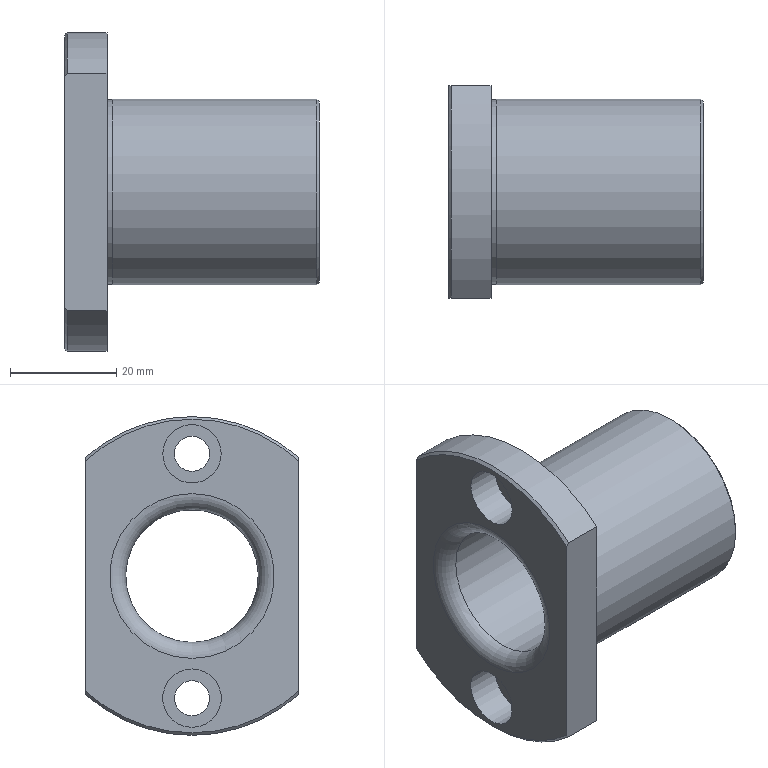Part | NX | features bushing 2 | 1 solid | 21 faces | box 48 x 40 x 60 mm | volume 31044 mm3 | cylinder 9 | plane 8 | cone 3 | torus 1 | commonest cylinder face diameters 6.6 x2 11 x2 60 x2 25 x1 34.65 x1 35 x1
STEP:
#1=CARTESIAN_POINT('',(-1.5,0.,-28.5));
#2=VERTEX_POINT('',#1);
#3=CARTESIAN_POINT('',(-1.5,0.,-23.));
#4=DIRECTION('',(1.,0.,0.));
#5=DIRECTION('',(0.,0.,-1.));
#6=AXIS2_PLACEMENT_3D('',#3,#4,#5);
#7=CIRCLE('',#6,5.5);
#8=EDGE_CURVE('',#2,#2,#7,.F.);
#9=ORIENTED_EDGE('',*,*,#8,.F.);
#10=EDGE_LOOP('',(#9));
#11=FACE_BOUND('',#10,.T.);
#12=CARTESIAN_POINT('',(-8.,0.,-28.5));
#13=VERTEX_POINT('',#12);
#14=CARTESIAN_POINT('',(-8.,0.,-23.));
#15=DIRECTION('',(1.,0.,0.));
#16=DIRECTION('',(0.,0.,-1.));
#17=AXIS2_PLACEMENT_3D('',#14,#15,#16);
#18=CIRCLE('',#17,5.5);
#19=EDGE_CURVE('',#13,#13,#18,.T.);
#20=ORIENTED_EDGE('',*,*,#19,.F.);
#21=EDGE_LOOP('',(#20));
#22=FACE_BOUND('',#21,.T.);
#23=CARTESIAN_POINT('',(-8.,0.,-23.));
#24=DIRECTION('',(1.,0.,0.));
#25=DIRECTION('',(0.,0.,-1.));
#26=AXIS2_PLACEMENT_3D('',#23,#24,#25);
#27=CYLINDRICAL_SURFACE('',#26,5.5);
#28=ADVANCED_FACE('',(#11,#22),#27,.F.);
#29=CARTESIAN_POINT('',(-1.5,5.5,23.));
#30=VERTEX_POINT('',#29);
#31=CARTESIAN_POINT('',(-1.5,0.,23.));
#32=DIRECTION('',(1.,0.,0.));
#33=DIRECTION('',(0.,1.,0.));
#34=AXIS2_PLACEMENT_3D('',#31,#32,#33);
#35=CIRCLE('',#34,5.5);
#36=EDGE_CURVE('',#30,#30,#35,.F.);
#37=ORIENTED_EDGE('',*,*,#36,.F.);
#38=EDGE_LOOP('',(#37));
#39=FACE_BOUND('',#38,.T.);
#40=CARTESIAN_POINT('',(-8.,5.5,23.));
#41=VERTEX_POINT('',#40);
#42=CARTESIAN_POINT('',(-8.,0.,23.));
#43=DIRECTION('',(1.,0.,0.));
#44=DIRECTION('',(0.,1.,0.));
#45=AXIS2_PLACEMENT_3D('',#42,#43,#44);
#46=CIRCLE('',#45,5.5);
#47=EDGE_CURVE('',#41,#41,#46,.T.);
#48=ORIENTED_EDGE('',*,*,#47,.F.);
#49=EDGE_LOOP('',(#48));
#50=FACE_BOUND('',#49,.T.);
#51=CARTESIAN_POINT('',(-8.,0.,23.));
#52=DIRECTION('',(1.,0.,0.));
#53=DIRECTION('',(0.,1.,0.));
#54=AXIS2_PLACEMENT_3D('',#51,#52,#53);
#55=CYLINDRICAL_SURFACE('',#54,5.5);
#56=ADVANCED_FACE('',(#39,#50),#55,.F.);
#57=CARTESIAN_POINT('',(-8.,-20.,21.685));
#58=VERTEX_POINT('',#57);
#59=CARTESIAN_POINT('',(-8.,20.,21.685));
#60=VERTEX_POINT('',#59);
#61=CARTESIAN_POINT('',(-8.,0.,0.));
#62=DIRECTION('',(-1.,0.,0.));
#63=DIRECTION('',(0.,0.,1.));
#64=AXIS2_PLACEMENT_3D('',#61,#62,#63);
#65=CIRCLE('',#64,29.5);
#66=EDGE_CURVE('',#58,#60,#65,.T.);
#67=ORIENTED_EDGE('',*,*,#66,.F.);
#68=CARTESIAN_POINT('',(-7.5,-20.,22.361));
#69=VERTEX_POINT('',#68);
#70=CARTESIAN_POINT('',(-8.,-20.,21.685));
#71=CARTESIAN_POINT('',(-7.834,-20.,21.911));
#72=CARTESIAN_POINT('',(-7.667,-20.,22.136));
#73=CARTESIAN_POINT('',(-7.5,-20.,22.361));
#74=B_SPLINE_CURVE_WITH_KNOTS('',3,(#70,#71,#72,#73),.UNSPECIFIED.,.F.,.F.,(4,4),(0.,0.0008404),.UNSPECIFIED.);
#75=EDGE_CURVE('',#58,#69,#74,.T.);
#76=ORIENTED_EDGE('',*,*,#75,.T.);
#77=CARTESIAN_POINT('',(-7.5,20.,22.361));
#78=VERTEX_POINT('',#77);
#79=CARTESIAN_POINT('',(-7.5,0.,0.));
#80=DIRECTION('',(1.,0.,0.));
#81=DIRECTION('',(0.,0.,-1.));
#82=AXIS2_PLACEMENT_3D('',#79,#80,#81);
#83=CIRCLE('',#82,30.);
#84=EDGE_CURVE('',#78,#69,#83,.T.);
#85=ORIENTED_EDGE('',*,*,#84,.F.);
#86=CARTESIAN_POINT('',(-8.,20.,21.685));
#87=CARTESIAN_POINT('',(-7.834,20.,21.911));
#88=CARTESIAN_POINT('',(-7.667,20.,22.136));
#89=CARTESIAN_POINT('',(-7.5,20.,22.361));
#90=B_SPLINE_CURVE_WITH_KNOTS('',3,(#86,#87,#88,#89),.UNSPECIFIED.,.F.,.F.,(4,4),(0.,0.0008404),.UNSPECIFIED.);
#91=EDGE_CURVE('',#60,#78,#90,.T.);
#92=ORIENTED_EDGE('',*,*,#91,.F.);
#93=EDGE_LOOP('',(#67,#76,#85,#92));
#94=FACE_BOUND('',#93,.T.);
#95=CARTESIAN_POINT('',(-7.5,0.,0.));
#96=DIRECTION('',(1.,0.,0.));
#97=DIRECTION('',(0.,0.,-1.));
#98=AXIS2_PLACEMENT_3D('',#95,#96,#97);
#99=CONICAL_SURFACE('',#98,30.,0.7854);
#100=ADVANCED_FACE('',(#94),#99,.T.);
#101=CARTESIAN_POINT('',(-8.,-20.,-21.685));
#102=VERTEX_POINT('',#101);
#103=CARTESIAN_POINT('',(-7.5,-20.,-22.361));
#104=VERTEX_POINT('',#103);
#105=CARTESIAN_POINT('',(-8.,-20.,-21.685));
#106=CARTESIAN_POINT('',(-7.834,-20.,-21.911));
#107=CARTESIAN_POINT('',(-7.667,-20.,-22.136));
#108=CARTESIAN_POINT('',(-7.5,-20.,-22.361));
#109=B_SPLINE_CURVE_WITH_KNOTS('',3,(#105,#106,#107,#108),.UNSPECIFIED.,.F.,.F.,(4,4),(0.,0.0008404),.UNSPECIFIED.);
#110=EDGE_CURVE('',#102,#104,#109,.T.);
#111=ORIENTED_EDGE('',*,*,#110,.F.);
#112=CARTESIAN_POINT('',(-8.,20.,-21.685));
#113=VERTEX_POINT('',#112);
#114=CARTESIAN_POINT('',(-8.,0.,0.));
#115=DIRECTION('',(1.,0.,0.));
#116=DIRECTION('',(0.,0.,-1.));
#117=AXIS2_PLACEMENT_3D('',#114,#115,#116);
#118=CIRCLE('',#117,29.5);
#119=EDGE_CURVE('',#113,#102,#118,.F.);
#120=ORIENTED_EDGE('',*,*,#119,.F.);
#121=CARTESIAN_POINT('',(-7.5,20.,-22.361));
#122=VERTEX_POINT('',#121);
#123=CARTESIAN_POINT('',(-7.5,20.,-22.361));
#124=CARTESIAN_POINT('',(-7.667,20.,-22.136));
#125=CARTESIAN_POINT('',(-7.834,20.,-21.911));
#126=CARTESIAN_POINT('',(-8.,20.,-21.685));
#127=B_SPLINE_CURVE_WITH_KNOTS('',3,(#123,#124,#125,#126),.UNSPECIFIED.,.F.,.F.,(4,4),(0.,0.0008404),.UNSPECIFIED.);
#128=EDGE_CURVE('',#122,#113,#127,.T.);
#129=ORIENTED_EDGE('',*,*,#128,.F.);
#130=CARTESIAN_POINT('',(-7.5,0.,0.));
#131=DIRECTION('',(1.,0.,0.));
#132=DIRECTION('',(0.,0.,-1.));
#133=AXIS2_PLACEMENT_3D('',#130,#131,#132);
#134=CIRCLE('',#133,30.);
#135=EDGE_CURVE('',#104,#122,#134,.T.);
#136=ORIENTED_EDGE('',*,*,#135,.F.);
#137=EDGE_LOOP('',(#111,#120,#129,#136));
#138=FACE_BOUND('',#137,.T.);
#139=CARTESIAN_POINT('',(-7.5,0.,0.));
#140=DIRECTION('',(1.,0.,0.));
#141=DIRECTION('',(0.,0.,-1.));
#142=AXIS2_PLACEMENT_3D('',#139,#140,#141);
#143=CONICAL_SURFACE('',#142,30.,0.7854);
#144=ADVANCED_FACE('',(#138),#143,.T.);
#145=CARTESIAN_POINT('',(-1.5,0.,-26.3));
#146=VERTEX_POINT('',#145);
#147=CARTESIAN_POINT('',(-1.5,0.,-23.));
#148=DIRECTION('',(1.,0.,0.));
#149=DIRECTION('',(0.,0.,-1.));
#150=AXIS2_PLACEMENT_3D('',#147,#148,#149);
#151=CIRCLE('',#150,3.3);
#152=EDGE_CURVE('',#146,#146,#151,.F.);
#153=ORIENTED_EDGE('',*,*,#152,.F.);
#154=EDGE_LOOP('',(#153));
#155=FACE_BOUND('',#154,.T.);
#156=ORIENTED_EDGE('',*,*,#8,.T.);
#157=EDGE_LOOP('',(#156));
#158=FACE_BOUND('',#157,.T.);
#159=CARTESIAN_POINT('',(-1.5,0.,-18.6));
#160=DIRECTION('',(-1.,0.,0.));
#161=DIRECTION('',(0.,0.,1.));
#162=AXIS2_PLACEMENT_3D('',#159,#160,#161);
#163=PLANE('',#162);
#164=ADVANCED_FACE('',(#155,#158),#163,.T.);
#165=CARTESIAN_POINT('',(-1.5,3.3,23.));
#166=VERTEX_POINT('',#165);
#167=CARTESIAN_POINT('',(-1.5,0.,23.));
#168=DIRECTION('',(1.,0.,0.));
#169=DIRECTION('',(0.,1.,0.));
#170=AXIS2_PLACEMENT_3D('',#167,#168,#169);
#171=CIRCLE('',#170,3.3);
#172=EDGE_CURVE('',#166,#166,#171,.F.);
#173=ORIENTED_EDGE('',*,*,#172,.F.);
#174=EDGE_LOOP('',(#173));
#175=FACE_BOUND('',#174,.T.);
#176=ORIENTED_EDGE('',*,*,#36,.T.);
#177=EDGE_LOOP('',(#176));
#178=FACE_BOUND('',#177,.T.);
#179=CARTESIAN_POINT('',(-1.5,0.,18.6));
#180=DIRECTION('',(-1.,0.,0.));
#181=DIRECTION('',(0.,-1.,0.));
#182=AXIS2_PLACEMENT_3D('',#179,#180,#181);
#183=PLANE('',#182);
#184=ADVANCED_FACE('',(#175,#178),#183,.T.);
#185=ORIENTED_EDGE('',*,*,#47,.T.);
#186=EDGE_LOOP('',(#185));
#187=FACE_BOUND('',#186,.T.);
#188=ORIENTED_EDGE('',*,*,#19,.T.);
#189=EDGE_LOOP('',(#188));
#190=FACE_BOUND('',#189,.T.);
#191=CARTESIAN_POINT('',(-8.,-20.,0.));
#192=DIRECTION('',(0.,0.,-1.));
#193=VECTOR('',#192,1000.);
#194=LINE('',#191,#193);
#195=EDGE_CURVE('',#58,#102,#194,.T.);
#196=ORIENTED_EDGE('',*,*,#195,.F.);
#197=ORIENTED_EDGE('',*,*,#66,.T.);
#198=CARTESIAN_POINT('',(-8.,20.,0.));
#199=DIRECTION('',(0.,0.,1.));
#200=VECTOR('',#199,1000.);
#201=LINE('',#198,#200);
#202=EDGE_CURVE('',#113,#60,#201,.T.);
#203=ORIENTED_EDGE('',*,*,#202,.F.);
#204=ORIENTED_EDGE('',*,*,#119,.T.);
#205=EDGE_LOOP('',(#196,#197,#203,#204));
#206=FACE_BOUND('',#205,.T.);
#207=CARTESIAN_POINT('',(-8.,0.,-15.5));
#208=VERTEX_POINT('',#207);
#209=CARTESIAN_POINT('',(-8.,0.,0.));
#210=DIRECTION('',(1.,0.,0.));
#211=DIRECTION('',(0.,0.,-1.));
#212=AXIS2_PLACEMENT_3D('',#209,#210,#211);
#213=CIRCLE('',#212,15.5);
#214=EDGE_CURVE('',#208,#208,#213,.F.);
#215=ORIENTED_EDGE('',*,*,#214,.F.);
#216=EDGE_LOOP('',(#215));
#217=FACE_BOUND('',#216,.T.);
#218=CARTESIAN_POINT('',(-8.,0.,14.75));
#219=DIRECTION('',(-1.,0.,0.));
#220=DIRECTION('',(0.,0.,1.));
#221=AXIS2_PLACEMENT_3D('',#218,#219,#220);
#222=PLANE('',#221);
#223=ADVANCED_FACE('',(#187,#190,#206,#217),#222,.T.);
#224=CARTESIAN_POINT('',(0.,20.,22.361));
#225=VERTEX_POINT('',#224);
#226=CARTESIAN_POINT('',(-3.75,20.,22.361));
#227=DIRECTION('',(1.,0.,0.));
#228=VECTOR('',#227,1000.);
#229=LINE('',#226,#228);
#230=EDGE_CURVE('',#225,#78,#229,.F.);
#231=ORIENTED_EDGE('',*,*,#230,.F.);
#232=CARTESIAN_POINT('',(0.,20.,-22.361));
#233=VERTEX_POINT('',#232);
#234=CARTESIAN_POINT('',(0.,20.,23.663));
#235=DIRECTION('',(0.,0.,1.));
#236=VECTOR('',#235,1000.);
#237=LINE('',#234,#236);
#238=EDGE_CURVE('',#233,#225,#237,.T.);
#239=ORIENTED_EDGE('',*,*,#238,.F.);
#240=CARTESIAN_POINT('',(-3.75,20.,-22.361));
#241=DIRECTION('',(1.,0.,0.));
#242=VECTOR('',#241,1000.);
#243=LINE('',#240,#242);
#244=EDGE_CURVE('',#122,#233,#243,.T.);
#245=ORIENTED_EDGE('',*,*,#244,.F.);
#246=ORIENTED_EDGE('',*,*,#128,.T.);
#247=ORIENTED_EDGE('',*,*,#202,.T.);
#248=ORIENTED_EDGE('',*,*,#91,.T.);
#249=EDGE_LOOP('',(#231,#239,#245,#246,#247,#248));
#250=FACE_BOUND('',#249,.T.);
#251=CARTESIAN_POINT('',(-4.,20.,0.));
#252=DIRECTION('',(0.,1.,0.));
#253=DIRECTION('',(0.,0.,1.));
#254=AXIS2_PLACEMENT_3D('',#251,#252,#253);
#255=PLANE('',#254);
#256=ADVANCED_FACE('',(#250),#255,.T.);
#257=CARTESIAN_POINT('',(0.,-20.,22.361));
#258=VERTEX_POINT('',#257);
#259=CARTESIAN_POINT('',(-4.,-20.,22.361));
#260=DIRECTION('',(1.,0.,0.));
#261=VECTOR('',#260,1000.);
#262=LINE('',#259,#261);
#263=EDGE_CURVE('',#258,#69,#262,.F.);
#264=ORIENTED_EDGE('',*,*,#263,.F.);
#265=CARTESIAN_POINT('',(0.,0.,0.));
#266=DIRECTION('',(1.,0.,0.));
#267=DIRECTION('',(0.,0.,-1.));
#268=AXIS2_PLACEMENT_3D('',#265,#266,#267);
#269=CIRCLE('',#268,30.);
#270=EDGE_CURVE('',#225,#258,#269,.T.);
#271=ORIENTED_EDGE('',*,*,#270,.F.);
#272=ORIENTED_EDGE('',*,*,#230,.T.);
#273=ORIENTED_EDGE('',*,*,#84,.T.);
#274=EDGE_LOOP('',(#264,#271,#272,#273));
#275=FACE_BOUND('',#274,.T.);
#276=CARTESIAN_POINT('',(-3.75,0.,0.));
#277=DIRECTION('',(1.,0.,0.));
#278=DIRECTION('',(0.,0.,-1.));
#279=AXIS2_PLACEMENT_3D('',#276,#277,#278);
#280=CYLINDRICAL_SURFACE('',#279,30.);
#281=ADVANCED_FACE('',(#275),#280,.T.);
#282=CARTESIAN_POINT('',(0.,-20.,-22.361));
#283=VERTEX_POINT('',#282);
#284=CARTESIAN_POINT('',(-3.75,-20.,-22.361));
#285=DIRECTION('',(1.,0.,0.));
#286=VECTOR('',#285,1000.);
#287=LINE('',#284,#286);
#288=EDGE_CURVE('',#283,#104,#287,.F.);
#289=ORIENTED_EDGE('',*,*,#288,.F.);
#290=CARTESIAN_POINT('',(0.,-20.,23.663));
#291=DIRECTION('',(0.,0.,1.));
#292=VECTOR('',#291,1000.);
#293=LINE('',#290,#292);
#294=EDGE_CURVE('',#258,#283,#293,.F.);
#295=ORIENTED_EDGE('',*,*,#294,.F.);
#296=ORIENTED_EDGE('',*,*,#263,.T.);
#297=ORIENTED_EDGE('',*,*,#75,.F.);
#298=ORIENTED_EDGE('',*,*,#195,.T.);
#299=ORIENTED_EDGE('',*,*,#110,.T.);
#300=EDGE_LOOP('',(#289,#295,#296,#297,#298,#299));
#301=FACE_BOUND('',#300,.T.);
#302=CARTESIAN_POINT('',(-4.,-20.,0.));
#303=DIRECTION('',(0.,-1.,0.));
#304=DIRECTION('',(0.,0.,-1.));
#305=AXIS2_PLACEMENT_3D('',#302,#303,#304);
#306=PLANE('',#305);
#307=ADVANCED_FACE('',(#301),#306,.T.);
#308=ORIENTED_EDGE('',*,*,#244,.T.);
#309=CARTESIAN_POINT('',(0.,0.,0.));
#310=DIRECTION('',(1.,0.,0.));
#311=DIRECTION('',(0.,0.,-1.));
#312=AXIS2_PLACEMENT_3D('',#309,#310,#311);
#313=CIRCLE('',#312,30.);
#314=EDGE_CURVE('',#283,#233,#313,.T.);
#315=ORIENTED_EDGE('',*,*,#314,.F.);
#316=ORIENTED_EDGE('',*,*,#288,.T.);
#317=ORIENTED_EDGE('',*,*,#135,.T.);
#318=EDGE_LOOP('',(#308,#315,#316,#317));
#319=FACE_BOUND('',#318,.T.);
#320=CARTESIAN_POINT('',(-3.75,0.,0.));
#321=DIRECTION('',(1.,0.,0.));
#322=DIRECTION('',(0.,0.,-1.));
#323=AXIS2_PLACEMENT_3D('',#320,#321,#322);
#324=CYLINDRICAL_SURFACE('',#323,30.);
#325=ADVANCED_FACE('',(#319),#324,.T.);
#326=ORIENTED_EDGE('',*,*,#152,.T.);
#327=EDGE_LOOP('',(#326));
#328=FACE_BOUND('',#327,.T.);
#329=CARTESIAN_POINT('',(0.,0.,-26.3));
#330=VERTEX_POINT('',#329);
#331=CARTESIAN_POINT('',(0.,0.,-23.));
#332=DIRECTION('',(1.,0.,0.));
#333=DIRECTION('',(0.,0.,-1.));
#334=AXIS2_PLACEMENT_3D('',#331,#332,#333);
#335=CIRCLE('',#334,3.3);
#336=EDGE_CURVE('',#330,#330,#335,.F.);
#337=ORIENTED_EDGE('',*,*,#336,.F.);
#338=EDGE_LOOP('',(#337));
#339=FACE_BOUND('',#338,.T.);
#340=CARTESIAN_POINT('',(-1.5,0.,-23.));
#341=DIRECTION('',(1.,0.,0.));
#342=DIRECTION('',(0.,0.,-1.));
#343=AXIS2_PLACEMENT_3D('',#340,#341,#342);
#344=CYLINDRICAL_SURFACE('',#343,3.3);
#345=ADVANCED_FACE('',(#328,#339),#344,.F.);
#346=ORIENTED_EDGE('',*,*,#172,.T.);
#347=EDGE_LOOP('',(#346));
#348=FACE_BOUND('',#347,.T.);
#349=CARTESIAN_POINT('',(0.,3.3,23.));
#350=VERTEX_POINT('',#349);
#351=CARTESIAN_POINT('',(0.,0.,23.));
#352=DIRECTION('',(1.,0.,0.));
#353=DIRECTION('',(0.,1.,0.));
#354=AXIS2_PLACEMENT_3D('',#351,#352,#353);
#355=CIRCLE('',#354,3.3);
#356=EDGE_CURVE('',#350,#350,#355,.F.);
#357=ORIENTED_EDGE('',*,*,#356,.F.);
#358=EDGE_LOOP('',(#357));
#359=FACE_BOUND('',#358,.T.);
#360=CARTESIAN_POINT('',(-1.5,0.,23.));
#361=DIRECTION('',(1.,0.,0.));
#362=DIRECTION('',(0.,1.,0.));
#363=AXIS2_PLACEMENT_3D('',#360,#361,#362);
#364=CYLINDRICAL_SURFACE('',#363,3.3);
#365=ADVANCED_FACE('',(#348,#359),#364,.F.);
#366=ORIENTED_EDGE('',*,*,#214,.T.);
#367=EDGE_LOOP('',(#366));
#368=FACE_BOUND('',#367,.T.);
#369=CARTESIAN_POINT('',(-5.,0.,12.5));
#370=VERTEX_POINT('',#369);
#371=CARTESIAN_POINT('',(-5.,0.,0.));
#372=DIRECTION('',(-1.,0.,0.));
#373=DIRECTION('',(0.,0.,1.));
#374=AXIS2_PLACEMENT_3D('',#371,#372,#373);
#375=CIRCLE('',#374,12.5);
#376=EDGE_CURVE('',#370,#370,#375,.T.);
#377=ORIENTED_EDGE('',*,*,#376,.F.);
#378=EDGE_LOOP('',(#377));
#379=FACE_BOUND('',#378,.T.);
#380=CARTESIAN_POINT('',(-5.,0.,0.));
#381=DIRECTION('',(1.,0.,0.));
#382=DIRECTION('',(0.,0.,-1.));
#383=AXIS2_PLACEMENT_3D('',#380,#381,#382);
#384=TOROIDAL_SURFACE('',#383,15.5,3.);
#385=ADVANCED_FACE('',(#368,#379),#384,.T.);
#386=ORIENTED_EDGE('',*,*,#356,.T.);
#387=EDGE_LOOP('',(#386));
#388=FACE_BOUND('',#387,.T.);
#389=ORIENTED_EDGE('',*,*,#336,.T.);
#390=EDGE_LOOP('',(#389));
#391=FACE_BOUND('',#390,.T.);
#392=CARTESIAN_POINT('',(0.,0.,-17.325));
#393=VERTEX_POINT('',#392);
#394=CARTESIAN_POINT('',(0.,0.,0.));
#395=DIRECTION('',(1.,0.,0.));
#396=DIRECTION('',(0.,0.,-1.));
#397=AXIS2_PLACEMENT_3D('',#394,#395,#396);
#398=CIRCLE('',#397,17.325);
#399=EDGE_CURVE('',#393,#393,#398,.T.);
#400=ORIENTED_EDGE('',*,*,#399,.F.);
#401=EDGE_LOOP('',(#400));
#402=FACE_BOUND('',#401,.T.);
#403=ORIENTED_EDGE('',*,*,#294,.T.);
#404=ORIENTED_EDGE('',*,*,#314,.T.);
#405=ORIENTED_EDGE('',*,*,#238,.T.);
#406=ORIENTED_EDGE('',*,*,#270,.T.);
#407=EDGE_LOOP('',(#403,#404,#405,#406));
#408=FACE_BOUND('',#407,.T.);
#409=CARTESIAN_POINT('',(0.,0.,23.663));
#410=DIRECTION('',(1.,0.,0.));
#411=DIRECTION('',(0.,1.,0.));
#412=AXIS2_PLACEMENT_3D('',#409,#410,#411);
#413=PLANE('',#412);
#414=ADVANCED_FACE('',(#388,#391,#402,#408),#413,.T.);
#415=ORIENTED_EDGE('',*,*,#376,.T.);
#416=EDGE_LOOP('',(#415));
#417=FACE_BOUND('',#416,.T.);
#418=CARTESIAN_POINT('',(40.,0.,-12.5));
#419=VERTEX_POINT('',#418);
#420=CARTESIAN_POINT('',(40.,0.,0.));
#421=DIRECTION('',(1.,0.,0.));
#422=DIRECTION('',(0.,0.,-1.));
#423=AXIS2_PLACEMENT_3D('',#420,#421,#422);
#424=CIRCLE('',#423,12.5);
#425=EDGE_CURVE('',#419,#419,#424,.F.);
#426=ORIENTED_EDGE('',*,*,#425,.F.);
#427=EDGE_LOOP('',(#426));
#428=FACE_BOUND('',#427,.T.);
#429=CARTESIAN_POINT('',(-5.,0.,0.));
#430=DIRECTION('',(1.,0.,0.));
#431=DIRECTION('',(0.,0.,-1.));
#432=AXIS2_PLACEMENT_3D('',#429,#430,#431);
#433=CYLINDRICAL_SURFACE('',#432,12.5);
#434=ADVANCED_FACE('',(#417,#428),#433,.F.);
#435=ORIENTED_EDGE('',*,*,#399,.T.);
#436=EDGE_LOOP('',(#435));
#437=FACE_BOUND('',#436,.T.);
#438=CARTESIAN_POINT('',(1.,0.,-17.325));
#439=VERTEX_POINT('',#438);
#440=CARTESIAN_POINT('',(1.,0.,0.));
#441=DIRECTION('',(1.,0.,0.));
#442=DIRECTION('',(0.,0.,-1.));
#443=AXIS2_PLACEMENT_3D('',#440,#441,#442);
#444=CIRCLE('',#443,17.325);
#445=EDGE_CURVE('',#439,#439,#444,.T.);
#446=ORIENTED_EDGE('',*,*,#445,.F.);
#447=EDGE_LOOP('',(#446));
#448=FACE_BOUND('',#447,.T.);
#449=CARTESIAN_POINT('',(0.5,0.,0.));
#450=DIRECTION('',(1.,0.,0.));
#451=DIRECTION('',(0.,0.,-1.));
#452=AXIS2_PLACEMENT_3D('',#449,#450,#451);
#453=CYLINDRICAL_SURFACE('',#452,17.325);
#454=ADVANCED_FACE('',(#437,#448),#453,.T.);
#455=ORIENTED_EDGE('',*,*,#425,.T.);
#456=EDGE_LOOP('',(#455));
#457=FACE_BOUND('',#456,.T.);
#458=CARTESIAN_POINT('',(40.,0.,17.));
#459=VERTEX_POINT('',#458);
#460=CARTESIAN_POINT('',(40.,0.,0.));
#461=DIRECTION('',(-1.,0.,0.));
#462=DIRECTION('',(0.,0.,1.));
#463=AXIS2_PLACEMENT_3D('',#460,#461,#462);
#464=CIRCLE('',#463,17.);
#465=EDGE_CURVE('',#459,#459,#464,.T.);
#466=ORIENTED_EDGE('',*,*,#465,.F.);
#467=EDGE_LOOP('',(#466));
#468=FACE_BOUND('',#467,.T.);
#469=CARTESIAN_POINT('',(40.,0.,8.5));
#470=DIRECTION('',(1.,0.,0.));
#471=DIRECTION('',(0.,1.,0.));
#472=AXIS2_PLACEMENT_3D('',#469,#470,#471);
#473=PLANE('',#472);
#474=ADVANCED_FACE('',(#457,#468),#473,.T.);
#475=CARTESIAN_POINT('',(1.,0.,-17.5));
#476=VERTEX_POINT('',#475);
#477=CARTESIAN_POINT('',(1.,0.,0.));
#478=DIRECTION('',(1.,0.,0.));
#479=DIRECTION('',(0.,0.,-1.));
#480=AXIS2_PLACEMENT_3D('',#477,#478,#479);
#481=CIRCLE('',#480,17.5);
#482=EDGE_CURVE('',#476,#476,#481,.T.);
#483=ORIENTED_EDGE('',*,*,#482,.F.);
#484=EDGE_LOOP('',(#483));
#485=FACE_BOUND('',#484,.T.);
#486=ORIENTED_EDGE('',*,*,#445,.T.);
#487=EDGE_LOOP('',(#486));
#488=FACE_BOUND('',#487,.T.);
#489=CARTESIAN_POINT('',(1.,0.,17.413));
#490=DIRECTION('',(-1.,0.,0.));
#491=DIRECTION('',(0.,0.,1.));
#492=AXIS2_PLACEMENT_3D('',#489,#490,#491);
#493=PLANE('',#492);
#494=ADVANCED_FACE('',(#485,#488),#493,.T.);
#495=CARTESIAN_POINT('',(39.5,0.,-17.5));
#496=VERTEX_POINT('',#495);
#497=CARTESIAN_POINT('',(39.5,0.,0.));
#498=DIRECTION('',(1.,0.,0.));
#499=DIRECTION('',(0.,0.,-1.));
#500=AXIS2_PLACEMENT_3D('',#497,#498,#499);
#501=CIRCLE('',#500,17.5);
#502=EDGE_CURVE('',#496,#496,#501,.F.);
#503=ORIENTED_EDGE('',*,*,#502,.F.);
#504=EDGE_LOOP('',(#503));
#505=FACE_BOUND('',#504,.T.);
#506=ORIENTED_EDGE('',*,*,#465,.T.);
#507=EDGE_LOOP('',(#506));
#508=FACE_BOUND('',#507,.T.);
#509=CARTESIAN_POINT('',(39.5,0.,0.));
#510=DIRECTION('',(-1.,0.,0.));
#511=DIRECTION('',(0.,0.,1.));
#512=AXIS2_PLACEMENT_3D('',#509,#510,#511);
#513=CONICAL_SURFACE('',#512,17.5,0.7854);
#514=ADVANCED_FACE('',(#505,#508),#513,.T.);
#515=ORIENTED_EDGE('',*,*,#502,.T.);
#516=EDGE_LOOP('',(#515));
#517=FACE_BOUND('',#516,.T.);
#518=ORIENTED_EDGE('',*,*,#482,.T.);
#519=EDGE_LOOP('',(#518));
#520=FACE_BOUND('',#519,.T.);
#521=CARTESIAN_POINT('',(20.25,0.,0.));
#522=DIRECTION('',(1.,0.,0.));
#523=DIRECTION('',(0.,0.,-1.));
#524=AXIS2_PLACEMENT_3D('',#521,#522,#523);
#525=CYLINDRICAL_SURFACE('',#524,17.5);
#526=ADVANCED_FACE('',(#517,#520),#525,.T.);
#527=CLOSED_SHELL('',(#28,#56,#100,#144,#164,#184,#223,#256,#281,#307,#325,#345,#365,#385,#414,#434,#454,#474,#494,#514,#526));
#528=MANIFOLD_SOLID_BREP('',#527);
#529=(LENGTH_UNIT()NAMED_UNIT(*)SI_UNIT(.MILLI.,.METRE.));
#530=UNCERTAINTY_MEASURE_WITH_UNIT(LENGTH_MEASURE(0.0508),#529,'','');
#531=(NAMED_UNIT(*)PLANE_ANGLE_UNIT()SI_UNIT($,.RADIAN.));
#532=(NAMED_UNIT(*)SI_UNIT($,.STERADIAN.)SOLID_ANGLE_UNIT());
#533=(GEOMETRIC_REPRESENTATION_CONTEXT(3)GLOBAL_UNCERTAINTY_ASSIGNED_CONTEXT((#530))GLOBAL_UNIT_ASSIGNED_CONTEXT((#529,#531,#532))REPRESENTATION_CONTEXT('',''));
#534=ADVANCED_BREP_SHAPE_REPRESENTATION('',(#528),#533);